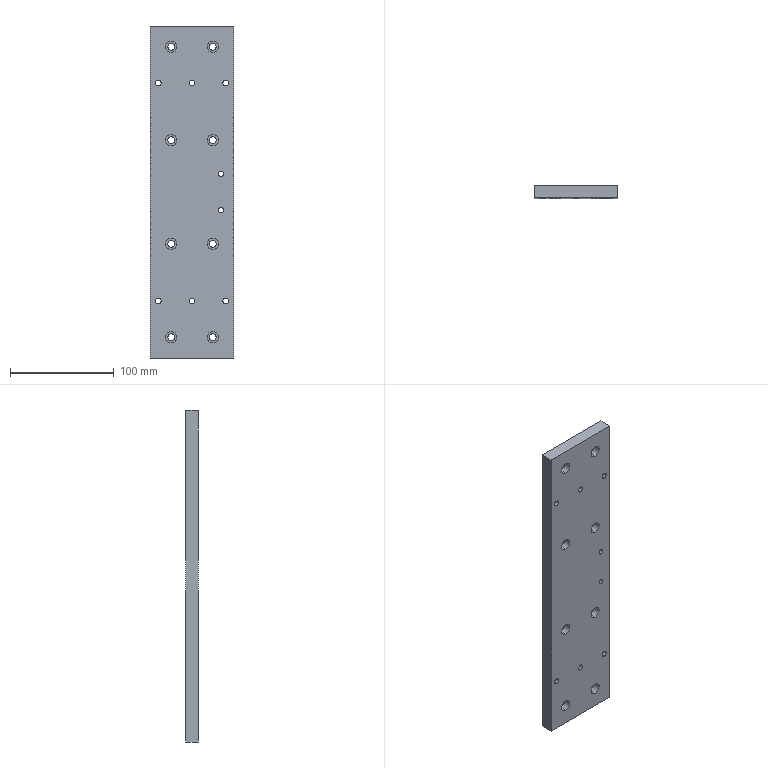Part | SolidWorks | features BaseBody 1 | 1 solid | 80 faces | box 80 x 12 x 320 mm | volume 296552 mm3 | cylinder 60 | plane 20 | commonest cylinder face diameters 6.6 x16 11 x16 5.5 x12 10 x12 5 x4